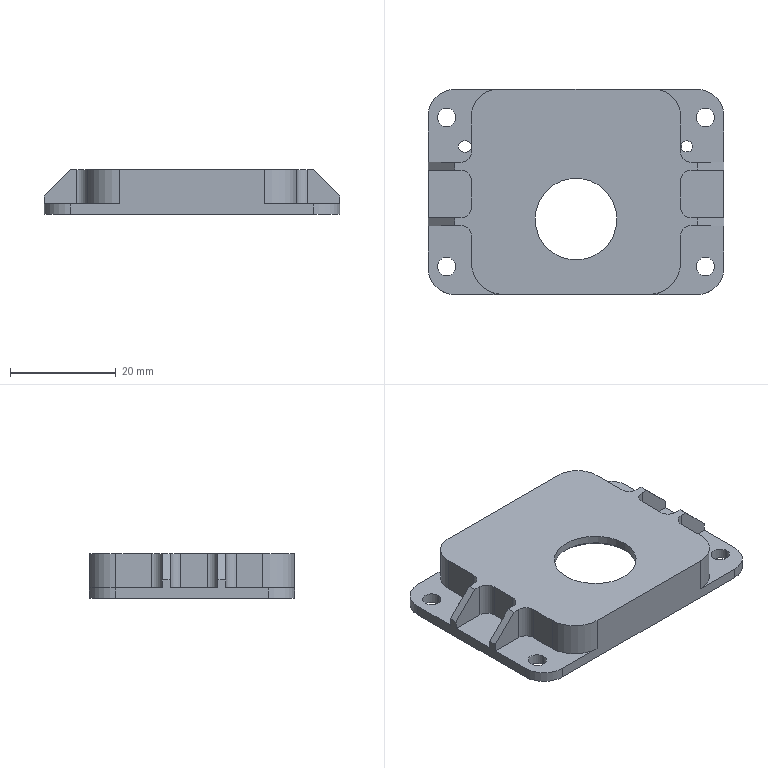NC program | NX | posted with a generic post | part box 56 x 38.85 x 8.5 mm
Lines 1 to 1050 of 4316:
N10 G17 G21 G94 G90
(FLOOR_WALL_COPY , TOOL : D80)
N12 T19 M6
N14 G54
N16 G17 G0 G90 X-75. Y0. S6500 M3
N18 G43 Z30. H19
N20 Z3.
N22 G94 G1 Z0. F1500.
N24 X-70.
N26 X70.
N28 X75.
N30 Z3.
N32 G0 Z30.
N34 M5
(ZLEVEL_PROFILE , TOOL : D10)
N36 T15 M6
N38 G54
N40 G17 G0 G90 X-33.1 Y6.668 S9500 M3
N42 G43 Z30. H15
N44 Z1.5
N46 G94 G1 Y15.204 Z1.053 F1000.
N48 X-32.737 Y17.218 Z0.945
N50 X-31.977 Y19.119 Z0.838
N52 X-30.85 Y20.828 Z0.731
N54 X-29.403 Y22.275 Z0.624
N56 X-27.694 Y23.402 Z0.516
N58 X-25.793 Y24.162 Z0.409
N60 X-23.779 Y24.525 Z0.302
N62 X0. Z-0.944
N64 X23. F3200.
N66 G2 X33.1 Y14.425 R10.1
N68 G1 Y-14.425
N70 G2 X23. Y-24.525 R10.1
N72 G1 X-23.
N74 G2 X-33.1 Y-14.425 R10.1
N76 G1 Y14.425
N78 G2 X-23. Y24.525 R10.1
N80 G1 X0.
N82 X22.416 Z-1.336
N84 X22.802 Z-1.342
N86 X23.189 Y24.523 Z-1.349
N88 X23.575 Y24.509 Z-1.356
N90 X23.96 Y24.479 Z-1.363
N92 X24.344 Y24.435 Z-1.369
N94 X24.726 Y24.376 Z-1.376
N96 X25.106 Y24.303 Z-1.383
N98 X25.482 Y24.215 Z-1.39
N100 X25.855 Y24.113 Z-1.396
N102 X26.223 Y23.997 Z-1.403
N104 X26.587 Y23.867 Z-1.41
N106 X26.946 Y23.722 Z-1.417
N108 X27.298 Y23.565 Z-1.423
N110 X27.645 Y23.394 Z-1.43
N112 X27.985 Y23.209 Z-1.437
N114 X28.317 Y23.012 Z-1.444
N116 X28.642 Y22.802 Z-1.45
N118 X28.958 Y22.58 Z-1.457
N120 X29.266 Y22.347 Z-1.464
N122 X29.564 Y22.101 Z-1.471
N124 X29.853 Y21.844 Z-1.477
N126 X30.132 Y21.577 Z-1.484
N128 X30.4 Y21.299 Z-1.491
N130 X30.658 Y21.011 Z-1.498
N132 X30.904 Y20.713 Z-1.504
N134 X31.139 Y20.406 Z-1.511
N136 X31.362 Y20.09 Z-1.518
N138 X31.572 Y19.766 Z-1.525
N140 X31.77 Y19.434 Z-1.531
N142 X31.956 Y19.095 Z-1.538
N144 X32.128 Y18.749 Z-1.545
N146 X32.286 Y18.397 Z-1.552
N148 X32.431 Y18.038 Z-1.558
N150 X32.563 Y17.675 Z-1.565
N152 X32.68 Y17.307 Z-1.572
N154 X32.783 Y16.934 Z-1.579
N156 X32.872 Y16.558 Z-1.585
N158 X32.947 Y16.179 Z-1.592
N160 X33.006 Y15.797 Z-1.599
N162 X33.052 Y15.413 Z-1.606
N164 X33.082 Y15.028 Z-1.612
N166 X33.098 Y14.642 Z-1.619
N168 X33.1 Y14.256 Z-1.626
N170 Y13.869 Z-1.633
N172 Y-0.817 Z-1.889
N174 Y-14.425
N176 G2 X23. Y-24.525 R10.1
N178 G1 X-23.
N180 G2 X-33.1 Y-14.425 R10.1
N182 G1 Y14.425
N184 G2 X-23. Y24.525 R10.1
N186 G1 X0.
N188 X22.416 Z-2.28
N190 X22.802 Z-2.287
N192 X23.189 Y24.523 Z-2.294
N194 X23.575 Y24.509 Z-2.3
N196 X23.96 Y24.479 Z-2.307
N198 X24.344 Y24.435 Z-2.314
N200 X24.726 Y24.376 Z-2.321
N202 X25.106 Y24.303 Z-2.327
N204 X25.482 Y24.215 Z-2.334
N206 X25.855 Y24.113 Z-2.341
N208 X26.223 Y23.997 Z-2.348
N210 X26.587 Y23.867 Z-2.354
N212 X26.946 Y23.722 Z-2.361
N214 X27.298 Y23.565 Z-2.368
N216 X27.645 Y23.394 Z-2.375
N218 X27.985 Y23.209 Z-2.381
N220 X28.317 Y23.012 Z-2.388
N222 X28.642 Y22.802 Z-2.395
N224 X28.958 Y22.58 Z-2.402
N226 X29.266 Y22.347 Z-2.408
N228 X29.564 Y22.101 Z-2.415
N230 X29.853 Y21.844 Z-2.422
N232 X30.132 Y21.577 Z-2.429
N234 X30.4 Y21.299 Z-2.435
N236 X30.658 Y21.011 Z-2.442
N238 X30.904 Y20.713 Z-2.449
N240 X31.139 Y20.406 Z-2.456
N242 X31.362 Y20.09 Z-2.462
N244 X31.572 Y19.766 Z-2.469
N246 X31.77 Y19.434 Z-2.476
N248 X31.956 Y19.095 Z-2.483
N250 X32.128 Y18.749 Z-2.489
N252 X32.286 Y18.397 Z-2.496
N254 X32.431 Y18.038 Z-2.503
N256 X32.563 Y17.675 Z-2.51
N258 X32.68 Y17.307 Z-2.516
N260 X32.783 Y16.934 Z-2.523
N262 X32.872 Y16.558 Z-2.53
N264 X32.947 Y16.179 Z-2.537
N266 X33.006 Y15.797 Z-2.543
N268 X33.052 Y15.413 Z-2.55
N270 X33.082 Y15.028 Z-2.557
N272 X33.098 Y14.642 Z-2.563
N274 X33.1 Y14.256 Z-2.57
N276 Y13.869 Z-2.577
N278 Y-0.817 Z-2.833
N280 Y-14.425
N282 G2 X23. Y-24.525 R10.1
N284 G1 X-23.
N286 G2 X-33.1 Y-14.425 R10.1
N288 G1 Y14.425
N290 G2 X-23. Y24.525 R10.1
N292 G1 X0.
N294 X22.416 Z-3.225
N296 X22.802 Z-3.231
N298 X23.189 Y24.523 Z-3.238
N300 X23.575 Y24.509 Z-3.245
N302 X23.96 Y24.479 Z-3.252
N304 X24.344 Y24.435 Z-3.258
N306 X24.726 Y24.376 Z-3.265
N308 X25.106 Y24.303 Z-3.272
N310 X25.482 Y24.215 Z-3.279
N312 X25.855 Y24.113 Z-3.285
N314 X26.223 Y23.997 Z-3.292
N316 X26.587 Y23.867 Z-3.299
N318 X26.946 Y23.722 Z-3.306
N320 X27.298 Y23.565 Z-3.312
N322 X27.645 Y23.394 Z-3.319
N324 X27.985 Y23.209 Z-3.326
N326 X28.317 Y23.012 Z-3.333
N328 X28.642 Y22.802 Z-3.339
N330 X28.958 Y22.58 Z-3.346
N332 X29.266 Y22.347 Z-3.353
N334 X29.564 Y22.101 Z-3.36
N336 X29.853 Y21.844 Z-3.366
N338 X30.132 Y21.577 Z-3.373
N340 X30.4 Y21.299 Z-3.38
N342 X30.658 Y21.011 Z-3.387
N344 X30.904 Y20.713 Z-3.393
N346 X31.139 Y20.406 Z-3.4
N348 X31.362 Y20.09 Z-3.407
N350 X31.572 Y19.766 Z-3.413
N352 X31.77 Y19.434 Z-3.42
N354 X31.956 Y19.095 Z-3.427
N356 X32.128 Y18.749 Z-3.434
N358 X32.286 Y18.397 Z-3.44
N360 X32.431 Y18.038 Z-3.447
N362 X32.563 Y17.675 Z-3.454
N364 X32.68 Y17.307 Z-3.461
N366 X32.783 Y16.934 Z-3.467
N368 X32.872 Y16.558 Z-3.474
N370 X32.947 Y16.179 Z-3.481
N372 X33.006 Y15.797 Z-3.488
N374 X33.052 Y15.413 Z-3.494
N376 X33.082 Y15.028 Z-3.501
N378 X33.098 Y14.642 Z-3.508
N380 X33.1 Y14.256 Z-3.515
N382 Y13.869 Z-3.521
N384 Y-0.817 Z-3.778
N386 Y-14.425
N388 G2 X23. Y-24.525 R10.1
N390 G1 X-23.
N392 G2 X-33.1 Y-14.425 R10.1
N394 G1 Y14.425
N396 G2 X-23. Y24.525 R10.1
N398 G1 X0.
N400 X22.416 Z-4.169
N402 X22.802 Z-4.176
N404 X23.189 Y24.523 Z-4.183
N406 X23.575 Y24.509 Z-4.189
N408 X23.96 Y24.479 Z-4.196
N410 X24.344 Y24.435 Z-4.203
N412 X24.726 Y24.376 Z-4.21
N414 X25.106 Y24.303 Z-4.216
N416 X25.482 Y24.215 Z-4.223
N418 X25.855 Y24.113 Z-4.23
N420 X26.223 Y23.997 Z-4.237
N422 X26.587 Y23.867 Z-4.243
N424 X26.946 Y23.722 Z-4.25
N426 X27.298 Y23.565 Z-4.257
N428 X27.645 Y23.394 Z-4.263
N430 X27.985 Y23.209 Z-4.27
N432 X28.317 Y23.012 Z-4.277
N434 X28.642 Y22.802 Z-4.284
N436 X28.958 Y22.58 Z-4.29
N438 X29.266 Y22.347 Z-4.297
N440 X29.564 Y22.101 Z-4.304
N442 X29.853 Y21.844 Z-4.311
N444 X30.132 Y21.577 Z-4.317
N446 X30.4 Y21.299 Z-4.324
N448 X30.658 Y21.011 Z-4.331
N450 X30.904 Y20.713 Z-4.338
N452 X31.139 Y20.406 Z-4.344
N454 X31.362 Y20.09 Z-4.351
N456 X31.572 Y19.766 Z-4.358
N458 X31.77 Y19.434 Z-4.365
N460 X31.956 Y19.095 Z-4.371
N462 X32.128 Y18.749 Z-4.378
N464 X32.286 Y18.397 Z-4.385
N466 X32.431 Y18.038 Z-4.392
N468 X32.563 Y17.675 Z-4.398
N470 X32.68 Y17.307 Z-4.405
N472 X32.783 Y16.934 Z-4.412
N474 X32.872 Y16.558 Z-4.419
N476 X32.947 Y16.179 Z-4.425
N478 X33.006 Y15.797 Z-4.432
N480 X33.052 Y15.413 Z-4.439
N482 X33.082 Y15.028 Z-4.446
N484 X33.098 Y14.642 Z-4.452
N486 X33.1 Y14.256 Z-4.459
N488 Y13.869 Z-4.466
N490 Y-0.817 Z-4.722
N492 Y-14.425
N494 G2 X23. Y-24.525 R10.1
N496 G1 X-23.
N498 G2 X-33.1 Y-14.425 R10.1
N500 G1 Y14.425
N502 G2 X-23. Y24.525 R10.1
N504 G1 X0.
N506 X22.416 Z-5.113
N508 X22.802 Z-5.12
N510 X23.189 Y24.523 Z-5.127
N512 X23.575 Y24.509 Z-5.134
N514 X23.96 Y24.479 Z-5.14
N516 X24.344 Y24.435 Z-5.147
N518 X24.726 Y24.376 Z-5.154
N520 X25.106 Y24.303 Z-5.161
N522 X25.482 Y24.215 Z-5.167
N524 X25.855 Y24.113 Z-5.174
N526 X26.223 Y23.997 Z-5.181
N528 X26.587 Y23.867 Z-5.188
N530 X26.946 Y23.722 Z-5.194
N532 X27.298 Y23.565 Z-5.201
N534 X27.645 Y23.394 Z-5.208
N536 X27.985 Y23.209 Z-5.215
N538 X28.317 Y23.012 Z-5.221
N540 X28.642 Y22.802 Z-5.228
N542 X28.958 Y22.58 Z-5.235
N544 X29.266 Y22.347 Z-5.242
N546 X29.564 Y22.101 Z-5.248
N548 X29.853 Y21.844 Z-5.255
N550 X30.132 Y21.577 Z-5.262
N552 X30.4 Y21.299 Z-5.269
N554 X30.658 Y21.011 Z-5.275
N556 X30.904 Y20.713 Z-5.282
N558 X31.139 Y20.406 Z-5.289
N560 X31.362 Y20.09 Z-5.296
N562 X31.572 Y19.766 Z-5.302
N564 X31.77 Y19.434 Z-5.309
N566 X31.956 Y19.095 Z-5.316
N568 X32.128 Y18.749 Z-5.323
N570 X32.286 Y18.397 Z-5.329
N572 X32.431 Y18.038 Z-5.336
N574 X32.563 Y17.675 Z-5.343
N576 X32.68 Y17.307 Z-5.35
N578 X32.783 Y16.934 Z-5.356
N580 X32.872 Y16.558 Z-5.363
N582 X32.947 Y16.179 Z-5.37
N584 X33.006 Y15.797 Z-5.377
N586 X33.052 Y15.413 Z-5.383
N588 X33.082 Y15.028 Z-5.39
N590 X33.098 Y14.642 Z-5.397
N592 X33.1 Y14.256 Z-5.404
N594 Y13.869 Z-5.41
N596 Y-0.817 Z-5.667
N598 Y-14.425
N600 G2 X23. Y-24.525 R10.1
N602 G1 X-23.
N604 G2 X-33.1 Y-14.425 R10.1
N606 G1 Y14.425
N608 G2 X-23. Y24.525 R10.1
N610 G1 X0.
N612 X22.416 Z-6.058
N614 X22.802 Z-6.065
N616 X23.189 Y24.523 Z-6.071
N618 X23.575 Y24.509 Z-6.078
N620 X23.96 Y24.479 Z-6.085
N622 X24.344 Y24.435 Z-6.092
N624 X24.726 Y24.376 Z-6.098
N626 X25.106 Y24.303 Z-6.105
N628 X25.482 Y24.215 Z-6.112
N630 X25.855 Y24.113 Z-6.119
N632 X26.223 Y23.997 Z-6.125
N634 X26.587 Y23.867 Z-6.132
N636 X26.946 Y23.722 Z-6.139
N638 X27.298 Y23.565 Z-6.146
N640 X27.645 Y23.394 Z-6.152
N642 X27.985 Y23.209 Z-6.159
N644 X28.317 Y23.012 Z-6.166
N646 X28.642 Y22.802 Z-6.173
N648 X28.958 Y22.58 Z-6.179
N650 X29.266 Y22.347 Z-6.186
N652 X29.564 Y22.101 Z-6.193
N654 X29.853 Y21.844 Z-6.2
N656 X30.132 Y21.577 Z-6.206
N658 X30.4 Y21.299 Z-6.213
N660 X30.658 Y21.011 Z-6.22
N662 X30.904 Y20.713 Z-6.227
N664 X31.139 Y20.406 Z-6.233
N666 X31.362 Y20.09 Z-6.24
N668 X31.572 Y19.766 Z-6.247
N670 X31.77 Y19.434 Z-6.254
N672 X31.956 Y19.095 Z-6.26
N674 X32.128 Y18.749 Z-6.267
N676 X32.286 Y18.397 Z-6.274
N678 X32.431 Y18.038 Z-6.281
N680 X32.563 Y17.675 Z-6.287
N682 X32.68 Y17.307 Z-6.294
N684 X32.783 Y16.934 Z-6.301
N686 X32.872 Y16.558 Z-6.308
N688 X32.947 Y16.179 Z-6.314
N690 X33.006 Y15.797 Z-6.321
N692 X33.052 Y15.413 Z-6.328
N694 X33.082 Y15.028 Z-6.335
N696 X33.098 Y14.642 Z-6.341
N698 X33.1 Y14.256 Z-6.348
N700 Y13.869 Z-6.355
N702 Y-0.817 Z-6.611
N704 Y-14.425
N706 G2 X23. Y-24.525 R10.1
N708 G1 X-23.
N710 G2 X-33.1 Y-14.425 R10.1
N712 G1 Y14.425
N714 G2 X-23. Y24.525 R10.1
N716 G1 X0.
N718 X22.416 Z-7.002
N720 X22.802 Z-7.009
N722 X23.189 Y24.523 Z-7.016
N724 X23.575 Y24.509 Z-7.023
N726 X23.96 Y24.479 Z-7.029
N728 X24.344 Y24.435 Z-7.036
N730 X24.726 Y24.376 Z-7.043
N732 X25.106 Y24.303 Z-7.05
N734 X25.482 Y24.215 Z-7.056
N736 X25.855 Y24.113 Z-7.063
N738 X26.223 Y23.997 Z-7.07
N740 X26.587 Y23.867 Z-7.077
N742 X26.946 Y23.722 Z-7.083
N744 X27.298 Y23.565 Z-7.09
N746 X27.645 Y23.394 Z-7.097
N748 X27.985 Y23.209 Z-7.104
N750 X28.317 Y23.012 Z-7.11
N752 X28.642 Y22.802 Z-7.117
N754 X28.958 Y22.58 Z-7.124
N756 X29.266 Y22.347 Z-7.131
N758 X29.564 Y22.101 Z-7.137
N760 X29.853 Y21.844 Z-7.144
N762 X30.132 Y21.577 Z-7.151
N764 X30.4 Y21.299 Z-7.158
N766 X30.658 Y21.011 Z-7.164
N768 X30.904 Y20.713 Z-7.171
N770 X31.139 Y20.406 Z-7.178
N772 X31.362 Y20.09 Z-7.185
N774 X31.572 Y19.766 Z-7.191
N776 X31.77 Y19.434 Z-7.198
N778 X31.956 Y19.095 Z-7.205
N780 X32.128 Y18.749 Z-7.212
N782 X32.286 Y18.397 Z-7.218
N784 X32.431 Y18.038 Z-7.225
N786 X32.563 Y17.675 Z-7.232
N788 X32.68 Y17.307 Z-7.238
N790 X32.783 Y16.934 Z-7.245
N792 X32.872 Y16.558 Z-7.252
N794 X32.947 Y16.179 Z-7.259
N796 X33.006 Y15.797 Z-7.265
N798 X33.052 Y15.413 Z-7.272
N800 X33.082 Y15.028 Z-7.279
N802 X33.098 Y14.642 Z-7.286
N804 X33.1 Y14.256 Z-7.292
N806 Y13.869 Z-7.299
N808 Y-0.817 Z-7.556
N810 Y-14.425
N812 G2 X23. Y-24.525 R10.1
N814 G1 X-23.
N816 G2 X-33.1 Y-14.425 R10.1
N818 G1 Y14.425
N820 G2 X-23. Y24.525 R10.1
N822 G1 X0.
N824 X22.416 Z-7.947
N826 X22.802 Z-7.954
N828 X23.189 Y24.523 Z-7.96
N830 X23.575 Y24.509 Z-7.967
N832 X23.96 Y24.479 Z-7.974
N834 X24.344 Y24.435 Z-7.981
N836 X24.726 Y24.376 Z-7.987
N838 X25.106 Y24.303 Z-7.994
N840 X25.482 Y24.215 Z-8.001
N842 X25.855 Y24.113 Z-8.008
N844 X26.223 Y23.997 Z-8.014
N846 X26.587 Y23.867 Z-8.021
N848 X26.946 Y23.722 Z-8.028
N850 X27.298 Y23.565 Z-8.035
N852 X27.645 Y23.394 Z-8.041
N854 X27.985 Y23.209 Z-8.048
N856 X28.317 Y23.012 Z-8.055
N858 X28.642 Y22.802 Z-8.062
N860 X28.958 Y22.58 Z-8.068
N862 X29.266 Y22.347 Z-8.075
N864 X29.564 Y22.101 Z-8.082
N866 X29.853 Y21.844 Z-8.088
N868 X30.132 Y21.577 Z-8.095
N870 X30.4 Y21.299 Z-8.102
N872 X30.658 Y21.011 Z-8.109
N874 X30.904 Y20.713 Z-8.115
N876 X31.139 Y20.406 Z-8.122
N878 X31.362 Y20.09 Z-8.129
N880 X31.572 Y19.766 Z-8.136
N882 X31.77 Y19.434 Z-8.142
N884 X31.956 Y19.095 Z-8.149
N886 X32.128 Y18.749 Z-8.156
N888 X32.286 Y18.397 Z-8.163
N890 X32.431 Y18.038 Z-8.169
N892 X32.563 Y17.675 Z-8.176
N894 X32.68 Y17.307 Z-8.183
N896 X32.783 Y16.934 Z-8.19
N898 X32.872 Y16.558 Z-8.196
N900 X32.947 Y16.179 Z-8.203
N902 X33.006 Y15.797 Z-8.21
N904 X33.052 Y15.413 Z-8.217
N906 X33.082 Y15.028 Z-8.223
N908 X33.098 Y14.642 Z-8.23
N910 X33.1 Y14.256 Z-8.237
N912 Y13.869 Z-8.244
N914 Y-0.817 Z-8.5
N916 Y-14.425
N918 G2 X23. Y-24.525 R10.1
N920 G1 X-23.
N922 G2 X-33.1 Y-14.425 R10.1
N924 G1 Y14.425
N926 G2 X-23. Y24.525 R10.1
N928 G1 X23.
N930 G2 X33.1 Y14.425 R10.1
N932 G1 Y-0.817
N934 Z-7.
N936 G0 Z30.
(HOLE_MILLING , TOOL : D10)
N938 X0. Y-5.148
N940 Z0.5
N942 G3 X1.325 Y-6.473 R1.325 F2000.
N944 X2.65 Y-5.148 R1.325
N946 X2.65 Y-5.148 Z-0.5 I-2.65 J0.
N948 X2.65 Y-5.148 Z-1.5 I-2.65 J0.
N950 X-2.65 Y-5.148 Z-2. I-2.65 J0.
N952 X0. Y-7.798 R2.65
N954 X-2.65 Y-5.148 R-2.65
N956 X-1.325 Y-6.473 R1.325
N958 X0. Y-5.148 R1.325
N960 G0 Z30.
(CAVITY_MILL , TOOL : D10)
N962 X-36.997 Y4.33
N964 Z0.086
N966 G1 Z-0.914 F1000.
N968 X-30.997 Y0.866
N970 G2 X-30.497 Y0. R1.
N972 G1 Y-21.043 F2500.
N974 G3 X-29.617 Y-21.922 R10.
N976 G1 X-22.693
N978 G3 X-19.304 Y-24.425 R12.3
N980 G1 X-15.287
N982 G2 X-24.9 Y-13.425 R11.1
N984 G1 Y-11.381
N986 G2 X-29.056 Y-6.375 R5.117
N988 G1 Y-4.875
N990 G2 X-26.337 Y-0.375 R5.103
N992 X-29.056 Y4.125 R5.097
N994 G1 Y5.625
N996 G2 X-24.9 Y10.628 R5.108
N998 G1 Y14.425
N1000 G2 X-16.218 Y24.425 R10.1
N1002 G1 X-20.062
N1004 G3 X-23.255 Y21.922 R11.3
N1006 G1 X-29.617
N1008 G3 X-30.497 Y21.043 R10.
N1010 G1 Y0.
N1012 G2 X-30.997 Y-0.866 R1.
N1014 G1 X-36.997 Y-4.33
N1016 Z0.086
N1018 G0 Y3.954 Z-0.829
N1020 G1 Z-1.829 F1000.
N1022 X-30.997 Y0.49
N1024 G2 X-30.497 Y-0.376 R1.
N1026 G1 Y-2.055 F2500.
N1028 G3 X-31.17 Y-4.875 R6.306
N1030 G1 Y-6.38
N1032 G3 X-30.497 Y-9.192 R6.316
N1034 G1 Y-21.043
N1036 G3 X-29.617 Y-21.923 R10.
N1038 G1 X-22.693
N1040 G3 X-19.304 Y-24.425 R12.3
N1042 G1 X-15.287
N1044 G2 X-24.9 Y-13.425 R11.1
N1046 G1 Y-11.471
N1048 G2 X-29.97 Y-6.375 R5.116
N1050 G1 Y-4.875
N1052 G2 X-27.251 Y-0.375 R5.106
N1054 X-29.97 Y4.125 R5.1
N1056 G1 Y5.625
N1058 G2 X-24.994 Y10.725 R5.127
N1060 G1 X-24.9
N1062 Y14.425
N1064 G2 X-16.218 Y24.425 R10.1
N1066 G1 X-20.062
N1068 G3 X-23.254 Y21.923 R11.3
N1070 G1 X-29.617
N1072 G3 X-30.497 Y21.043 R10.
N1074 G1 Y8.44
N1076 G3 X-31.17 Y5.625 R6.327
N1078 G1 Y4.123
N1080 G3 X-30.497 Y1.302 R6.3
N1082 G1 Y-0.376
N1084 G2 X-30.997 Y-1.242 R1.
N1086 G1 X-36.997 Y-4.706
N1088 Z-0.829
N1090 G0 X-36.998 Y3.954 Z-1.743
N1092 G1 Z-2.743 F1000.
N1094 X-30.998 Y0.49
N1096 G2 X-30.498 Y-0.376 R1.
N1098 G1 Y-0.706 F2500.
N1100 G3 X-32.084 Y-4.875 R6.304
N1102 G1 Y-6.38
N1104 G3 X-30.498 Y-10.543 R6.321
N1106 G1 Y-21.042
N1108 G3 X-29.617 Y-21.923 R10.
N1110 G1 X-22.692
N1112 G3 X-19.304 Y-24.425 R12.3
N1114 G1 X-15.287
N1116 G2 X-24.9 Y-13.425 R11.1
N1118 G1 Y-11.475
N1120 X-25.743
N1122 G2 X-30.884 Y-6.375 R5.121
N1124 G1 Y-4.875
N1126 G2 X-28.165 Y-0.375 R5.104
N1128 X-30.884 Y4.125 R5.099
N1130 G1 Y5.625
N1132 G2 X-25.743 Y10.725 R5.121
N1134 G1 X-24.9
N1136 Y14.425
N1138 G2 X-16.218 Y24.425 R10.1
N1140 G1 X-20.062
N1142 G3 X-23.254 Y21.923 R11.3
N1144 G1 X-29.617
N1146 G3 X-30.498 Y21.042 R10.
N1148 G1 Y9.793
N1150 G3 X-32.084 Y5.625 R6.321
N1152 G1 Y4.123
N1154 G3 X-30.498 Y-0.046 R6.299
N1156 G1 Y-0.376
N1158 G2 X-30.998 Y-1.242 R1.
N1160 G1 X-36.998 Y-4.706
N1162 Z-1.743
N1164 G0 Y0.587 Z-2.657
N1166 G1 Z-3.657 F1000.
N1168 X-30.826
N1170 G2 X-31.097 Y-0.376 R1.
N1172 G3 X-32.999 Y-4.875 R6.307 F2500.
N1174 G1 Y-6.38
N1176 G3 X-30.498 Y-11.39 R6.321
N1178 G1 Y-21.042
N1180 G3 X-29.616 Y-21.923 R10.
N1182 G1 X-22.692
N1184 G3 X-19.304 Y-24.425 R12.3
N1186 G1 X-15.287
N1188 G2 X-24.9 Y-13.425 R11.1
N1190 G1 Y-11.475
N1192 X-26.657
N1194 G2 X-31.799 Y-6.375 R5.121
N1196 G1 Y-4.875
N1198 G2 X-29.08 Y-0.375 R5.107
N1200 X-31.799 Y4.125 R5.101
N1202 G1 Y5.625
N1204 G2 X-26.657 Y10.725 R5.121
N1206 G1 X-24.9
N1208 Y11.925
N1210 Y14.425
N1212 G2 X-16.218 Y24.425 R10.1
N1214 G1 X-20.062
N1216 G3 X-23.254 Y21.923 R11.3
N1218 G1 X-29.616
N1220 G3 X-30.498 Y21.042 R10.
N1222 G1 Y10.64
N1224 G3 X-32.999 Y5.625 R6.321
N1226 G1 Y4.123
N1228 G3 X-31.097 Y-0.376 R6.301
N1230 G2 X-30.826 Y-1.338 R1.
N1232 G1 X-36.998
N1234 Z-2.657
N1236 G0 Y0.587 Z-3.571
N1238 G1 Z-4.571 F1000.
N1240 X-31.74
N1242 G2 X-32.011 Y-0.375 R1.
N1244 G1 X-30.883 Y-0.652
N1246 X-30.73 Y-0.85
N1248 G2 X-29.994 Y-0.375 R5.106 F2500.
N1250 X-32.713 Y4.125 R5.104
N1252 G1 Y5.625
N1254 G2 X-27.571 Y10.725 R5.16
N1256 G1 X-24.9
N1258 Y11.925
N1260 Y14.425
N1262 G2 X-16.218 Y24.425 R10.1
N1264 G1 X-20.062
N1266 G3 X-23.253 Y21.924 R11.3
N1268 G1 X-29.616
N1270 G3 X-30.498 Y21.041 R10.
N1272 G1 Y11.202
N1274 G3 X-33. Y8.848 R6.36
N1276 G1 Y0.87
N1278 G3 X-32.011 Y-0.375 R6.304
N1280 X-33. Y-1.621 R6.306
N1282 G1 Y-9.664
N1284 G3 X-30.601 Y-11.907 R6.185
N1286 G1 X-30.498 Y-11.96
N1288 Y-21.041
N1290 G3 X-29.616 Y-21.924 R10.
N1292 G1 X-22.692
N1294 G3 X-19.304 Y-24.425 R12.3
N1296 G1 X-15.287
N1298 G2 X-24.9 Y-13.425 R11.1
N1300 G1 Y-11.475
N1302 X-27.571
N1304 G2 X-30.043 Y-10.844 R5.518
N1306 X-32.713 Y-6.429 R4.985
N1308 G1 Y-4.875
N1310 G2 X-30.73 Y-0.85 R5.106
N1312 G3 X-30.541 Y-0.387 R0.5
N1314 G1 X-36.998
N1316 Z-3.571
N1318 G0 X-36.999 Y10.93 Z-4.486
N1320 G1 Z-5.486 F1000.
N1322 X-33.5 Y8.91
N1324 G2 X-33. Y8.044 R1.
N1326 G1 Y6.63 F2500.
N1328 G2 X-28. Y10.725 R5.1
N1330 G1 X-24.9
N1332 Y14.425
N1334 G2 X-16.218 Y24.425 R10.1
N1336 G1 X-20.062
N1338 G3 X-23.253 Y21.924 R11.3
N1340 G1 X-29.616
N1342 G3 X-30.499 Y21.041 R10.
N1344 G1 Y11.408
N1346 G3 X-33. Y9.458 R6.3
N1348 G1 Y8.044
N1350 G2 X-33.5 Y7.178 R1.
N1352 G1 X-36.999 Y5.158
N1354 Z-4.486
N1356 G0 Y10.93 Z-5.4
N1358 G1 Z-6.4 F1000.
N1360 X-33.5 Y8.91
N1362 G2 X-33. Y8.044 R1.
N1364 G1 Y6.63 F2500.
N1366 G2 X-28. Y10.725 R5.1
N1368 G1 X-24.9
N1370 Y14.425
N1372 G2 X-16.218 Y24.425 R10.1
N1374 G1 X-20.062
N1376 G3 X-23.253 Y21.924 R11.3
N1378 G1 X-29.615
N1380 G3 X-30.499 Y21.04 R10.
N1382 G1 Y11.408
N1384 G3 X-33. Y9.458 R6.3
N1386 G1 Y8.044
N1388 G2 X-33.5 Y7.178 R1.
N1390 G1 X-36.999 Y5.158
N1392 Z-5.4
N1394 G0 Z30.
N1396 Y0.474
N1398 Z-4.486
N1400 G1 Z-5.486 F1000.
N1402 X-33.5
N1404 G2 X-33. Y-0.392 R1.
N1406 G1 Y-3.87 F2500.
N1408 G2 X-30.432 Y-0.392 R5.1
N1410 X-33. Y3.085 R5.1
N1412 G1 Y-0.392
N1414 G2 X-33.5 Y-1.258 R1.
N1416 G1 X-36.999
N1418 Z-4.486
N1420 G0 Y0.474 Z-5.4
N1422 G1 Z-6.4 F1000.
N1424 X-33.5
N1426 G2 X-33. Y-0.392 R1.
N1428 G1 Y-3.87 F2500.
N1430 G2 X-30.432 Y-0.392 R5.1
N1432 X-33. Y3.085 R5.1
N1434 G1 Y-0.392
N1436 G2 X-33.5 Y-1.258 R1.
N1438 G1 X-36.999
N1440 Z-5.4
N1442 G0 Z30.
N1444 Y-12.269
N1446 Z-4.486
N1448 G1 Z-5.486 F1000.
N1450 X-30.999 Y-15.734
N1452 G2 X-30.499 Y-16.6 R1.
N1454 G1 Y-21.041 F2500.
N1456 G3 X-29.616 Y-21.924 R10.
N1458 G1 X-22.691
N1460 G3 X-19.304 Y-24.425 R12.3
N1462 G1 X-15.287
N1464 G2 X-24.9 Y-13.425 R11.1
N1466 G1 Y-11.475
N1468 X-28.
N1470 G2 X-33. Y-7.38 R5.1
N1472 G1 Y-10.208
N1474 G3 X-30.499 Y-12.158 R6.3
N1476 G1 Y-16.6
N1478 G2 X-30.999 Y-17.466 R1.
N1480 G1 X-36.619 Y-20.711
N1482 Z-4.486
N1484 G0 X-36.999 Y-12.269 Z-5.4
N1486 G1 Z-6.4 F1000.
N1488 X-30.999 Y-15.733
N1490 G2 X-30.499 Y-16.599 R1.
N1492 G1 Y-21.04 F2500.
N1494 G3 X-29.615 Y-21.924 R10.
N1496 G1 X-22.691
N1498 G3 X-19.304 Y-24.425 R12.3
N1500 G1 X-15.287
N1502 G2 X-24.9 Y-13.425 R11.1
N1504 G1 Y-11.475
N1506 X-28.
N1508 G2 X-33. Y-7.38 R5.1
N1510 G1 Y-10.208
N1512 G3 X-30.499 Y-12.158 R6.3
N1514 G1 Y-16.599
N1516 G2 X-30.999 Y-17.465 R1.
N1518 G1 X-36.62 Y-20.71
N1520 Z-5.4
N1522 G0 Z30.
N1524 X36.997 Y-4.33
N1526 Z0.086
N1528 G1 Z-0.914 F1000.
N1530 X30.997 Y-0.866
N1532 G2 X30.497 Y0. R1.
N1534 G1 Y21.043 F2500.
N1536 G3 X29.617 Y21.922 R10.
N1538 G1 X23.255
N1540 G3 X20.062 Y24.425 R11.3
N1542 G1 X16.218
N1544 G2 X24.9 Y14.425 R10.1
N1546 G1 Y10.628
N1548 G2 X29.056 Y5.625 R5.108
N1550 G1 Y4.125
N1552 G2 X26.337 Y-0.375 R5.096
N1554 X29.056 Y-4.875 R5.103
N1556 G1 Y-6.375
N1558 G2 X24.9 Y-11.381 R5.117
N1560 G1 Y-13.425
N1562 G2 X15.287 Y-24.425 R11.1
N1564 G1 X19.304
N1566 G3 X22.693 Y-21.922 R12.3
N1568 G1 X29.617
N1570 G3 X30.497 Y-21.043 R10.
N1572 G1 Y0.
N1574 G2 X30.997 Y0.866 R1.
N1576 G1 X36.997 Y4.33
N1578 Z0.086
N1580 G0 Y-4.706 Z-0.829
N1582 G1 Z-1.829 F1000.
N1584 X30.997 Y-1.242
N1586 G2 X30.497 Y-0.376 R1.
N1588 G1 Y1.303 F2500.
N1590 G3 X31.17 Y4.125 R6.301
N1592 G1 Y5.637
N1594 G3 X30.497 Y8.42 R6.355
N1596 G1 Y21.043
N1598 G3 X29.617 Y21.923 R10.
N1600 G1 X23.254
N1602 G3 X20.062 Y24.425 R11.3
N1604 G1 X16.218
N1606 G2 X24.9 Y14.425 R10.1
N1608 G1 Y10.725
N1610 X24.994
N1612 G2 X29.97 Y5.625 R5.155
N1614 G1 Y4.125
N1616 G2 X27.251 Y-0.375 R5.101
N1618 X29.97 Y-4.875 R5.104
N1620 G1 Y-6.375
N1622 G2 X24.9 Y-11.471 R5.116
N1624 G1 Y-13.425
N1626 G2 X15.287 Y-24.425 R11.1
N1628 G1 X19.304
N1630 G3 X22.693 Y-21.923 R12.3
N1632 G1 X29.617
N1634 G3 X30.497 Y-21.043 R10.
N1636 G1 Y-9.192
N1638 G3 X31.17 Y-6.375 R6.316
N1640 G1 Y-4.872
N1642 G3 X30.497 Y-2.054 R6.304
N1644 G1 Y-0.376
N1646 G2 X30.997 Y0.491 R1.
N1648 G1 X36.997 Y3.955
N1650 Z-0.829
N1652 G0 X36.998 Y-4.705 Z-1.743
N1654 G1 Z-2.743 F1000.
N1656 X30.998 Y-1.241
N1658 G2 X30.498 Y-0.375 R1.
N1660 G1 Y-0.045 F2500.
N1662 G3 X32.084 Y4.125 R6.3
N1664 G1 Y5.63
N1666 G3 X30.498 Y9.793 R6.321
N1668 G1 Y21.042
N1670 G3 X29.617 Y21.923 R10.
N1672 G1 X23.254
N1674 G3 X20.062 Y24.425 R11.3
N1676 G1 X16.218
N1678 G2 X24.9 Y14.425 R10.1
N1680 G1 Y10.725
N1682 X25.743
N1684 G2 X30.884 Y5.625 R5.121
N1686 G1 Y4.125
N1688 G2 X28.165 Y-0.375 R5.1
N1690 X30.884 Y-4.875 R5.102
N1692 G1 Y-6.375
N1694 G2 X25.743 Y-11.475 R5.121
N1696 G1 X24.9
N1698 Y-13.425
N1700 G2 X15.287 Y-24.425 R11.1
N1702 G1 X19.304
N1704 G3 X22.692 Y-21.923 R12.3
N1706 G1 X29.617
N1708 G3 X30.498 Y-21.042 R10.
N1710 G1 Y-10.543
N1712 G3 X32.084 Y-6.375 R6.321
N1714 G1 Y-4.872
N1716 G3 X30.498 Y-0.705 R6.302
N1718 G1 Y-0.375
N1720 G2 X30.998 Y0.491 R1.
N1722 G1 X36.998 Y3.955
N1724 Z-1.743
N1726 G0 Y-1.338 Z-2.657
N1728 G1 Z-3.657 F1000.
N1730 X30.826
N1732 G2 X31.097 Y-0.375 R1.
N1734 G3 X32.999 Y4.125 R6.301 F2500.
N1736 G1 Y5.63
N1738 G3 X30.498 Y10.64 R6.321
N1740 G1 Y21.042
N1742 G3 X29.616 Y21.923 R10.
N1744 G1 X23.254
N1746 G3 X20.062 Y24.425 R11.3
N1748 G1 X16.218
N1750 G2 X24.9 Y14.425 R10.1
N1752 G1 Y10.725
N1754 X26.657
N1756 G2 X31.799 Y5.625 R5.121
N1758 G1 Y4.125
N1760 G2 X29.08 Y-0.375 R5.101
N1762 X31.799 Y-4.875 R5.107
N1764 G1 Y-6.375
N1766 G2 X26.657 Y-11.475 R5.121
N1768 G1 X24.9
N1770 Y-13.425
N1772 G2 X15.287 Y-24.425 R11.1
N1774 G1 X19.304
N1776 G3 X22.692 Y-21.923 R12.3
N1778 G1 X29.616
N1780 G3 X30.498 Y-21.042 R10.
N1782 G1 Y-11.39
N1784 G3 X32.999 Y-6.375 R6.321
N1786 G1 Y-4.872
N1788 G3 X31.097 Y-0.375 R6.307
N1790 G2 X30.826 Y0.587 R1.
N1792 G1 X36.998
N1794 Z-2.657
N1796 G0 Y-1.338 Z-3.571
N1798 G1 Z-4.571 F1000.
N1800 X31.74
N1802 G2 X32.01 Y-0.376 R1.
N1804 G1 X30.883 Y-0.652
N1806 X30.73 Y-0.85
N1808 G2 X32.713 Y-4.875 R5.11 F2500.
N1810 G1 Y-6.385
N1812 G2 X28.662 Y-11.339 R5.055
N1814 X27.571 Y-11.475 R7.229
N1816 G1 X24.9
N1818 Y-13.425
N1820 G2 X15.287 Y-24.425 R11.1
N1822 G1 X19.304
N1824 G3 X22.692 Y-21.924 R12.3
N1826 G1 X29.616
N1828 G3 X30.498 Y-21.041 R10.
N1830 G1 Y-11.958
N1832 G3 X33. Y-9.639 R6.255
N1834 G1 Y-1.622
N1836 G3 X32.01 Y-0.376 R6.31
N1838 X33. Y0.87 R6.303
N1840 G1 Y8.848
N1842 G3 X30.498 Y11.202 R6.36
N1844 G1 Y21.041
N1846 G3 X29.616 Y21.924 R10.
N1848 G1 X23.253
N1850 G3 X20.062 Y24.425 R11.3
N1852 G1 X16.218
N1854 G2 X24.9 Y14.425 R10.1
N1856 G1 Y10.725
N1858 X27.571
N1860 G2 X32.713 Y5.625 R5.16
N1862 G1 Y4.125
N1864 G2 X29.994 Y-0.375 R5.103
N1866 X30.73 Y-0.85 R5.11
N1868 G3 X31.721 Y-0.984 R1.
N1870 G1 X36.998 Y1.177
N1872 Z-3.571
N1874 G0 X36.999 Y-11.68 Z-4.486
N1876 G1 Z-5.486 F1000.
N1878 X33.5 Y-9.66
N1880 G2 X33. Y-8.794 R1.
N1882 G1 Y-7.38 F2500.
N1884 G2 X28. Y-11.475 R5.1
N1886 G1 X24.9
N1888 Y-13.425
N1890 G2 X15.287 Y-24.425 R11.1
N1892 G1 X19.304
N1894 G3 X22.691 Y-21.924 R12.3
N1896 G1 X29.616
N1898 G3 X30.499 Y-21.041 R10.
N1900 G1 Y-12.158
N1902 G3 X33. Y-10.208 R6.3
N1904 G1 Y-8.794
N1906 G2 X33.5 Y-7.928 R1.
N1908 G1 X36.999 Y-5.908
N1910 Z-4.486
N1912 G0 Y-11.68 Z-5.4
N1914 G1 Z-6.4 F1000.
N1916 X33.5 Y-9.66
N1918 G2 X33. Y-8.794 R1.
N1920 G1 Y-7.38 F2500.
N1922 G2 X28. Y-11.475 R5.1
N1924 G1 X24.9
N1926 Y-13.425
N1928 G2 X15.287 Y-24.425 R11.1
N1930 G1 X19.304
N1932 G3 X22.691 Y-21.924 R12.3
N1934 G1 X29.615
N1936 G3 X30.499 Y-21.04 R10.
N1938 G1 Y-12.158
N1940 G3 X33. Y-10.208 R6.3
N1942 G1 Y-8.794
N1944 G2 X33.5 Y-7.928 R1.
N1946 G1 X36.999 Y-5.908
N1948 Z-5.4
N1950 G0 Z30.
N1952 Y-1.252
N1954 Z-4.486
N1956 G1 Z-5.486 F1000.
N1958 X33.5
N1960 G2 X33. Y-0.386 R1.
N1962 G1 Y3.098 F2500.
N1964 G2 X30.436 Y-0.394 R5.134
N1966 X33. Y-3.87 R5.1
N1968 G1 Y-0.386
N1970 G2 X33.5 Y0.48 R1.
N1972 G1 X36.999
N1974 Z-4.486
N1976 G0 Y-1.252 Z-5.4
N1978 G1 Z-6.4 F1000.
N1980 X33.5
N1982 G2 X33. Y-0.386 R1.
N1984 G1 Y3.098 F2500.
N1986 G2 X30.436 Y-0.394 R5.134
N1988 X33. Y-3.87 R5.1
N1990 G1 Y-0.386
N1992 G2 X33.5 Y0.48 R1.
N1994 G1 X36.999
N1996 Z-5.4
N1998 G0 Z30.
N2000 Y11.894
N2002 Z-4.486
N2004 G1 Z-5.486 F1000.
N2006 X30.999 Y15.359
N2008 G2 X30.499 Y16.225 R1.
N2010 G1 Y21.041 F2500.
N2012 G3 X29.616 Y21.924 R10.
N2014 G1 X23.253
N2016 G3 X20.062 Y24.425 R11.3
N2018 G1 X16.218
N2020 G2 X24.9 Y14.425 R10.1
N2022 G1 Y10.725
N2024 X28.
N2026 G2 X33. Y6.63 R5.1
N2028 G1 Y9.458
N2030 G3 X30.499 Y11.408 R6.3
N2032 G1 Y16.225
N2034 G2 X30.999 Y17.091 R1.
N2036 G1 X36.753 Y20.413
N2038 Z-4.486
N2040 G0 X36.999 Y11.894 Z-5.4
N2042 G1 Z-6.4 F1000.
N2044 X30.999 Y15.358
N2046 G2 X30.499 Y16.224 R1.
N2048 G1 Y21.04 F2500.
N2050 G3 X29.615 Y21.924 R10.
N2052 G1 X23.253
N2054 G3 X20.062 Y24.425 R11.3
N2056 G1 X16.218
N2058 G2 X24.9 Y14.425 R10.1
N2060 G1 Y10.725
N2062 X28.
N2064 G2 X33. Y6.63 R5.1
N2066 G1 Y9.458
N2068 G3 X30.499 Y11.408 R6.3
N2070 G1 Y16.224
N2072 G2 X30.999 Y17.09 R1.
N2074 G1 X36.753 Y20.412
N2076 Z-5.4
N2078 G0 Z30.
N2080 M5